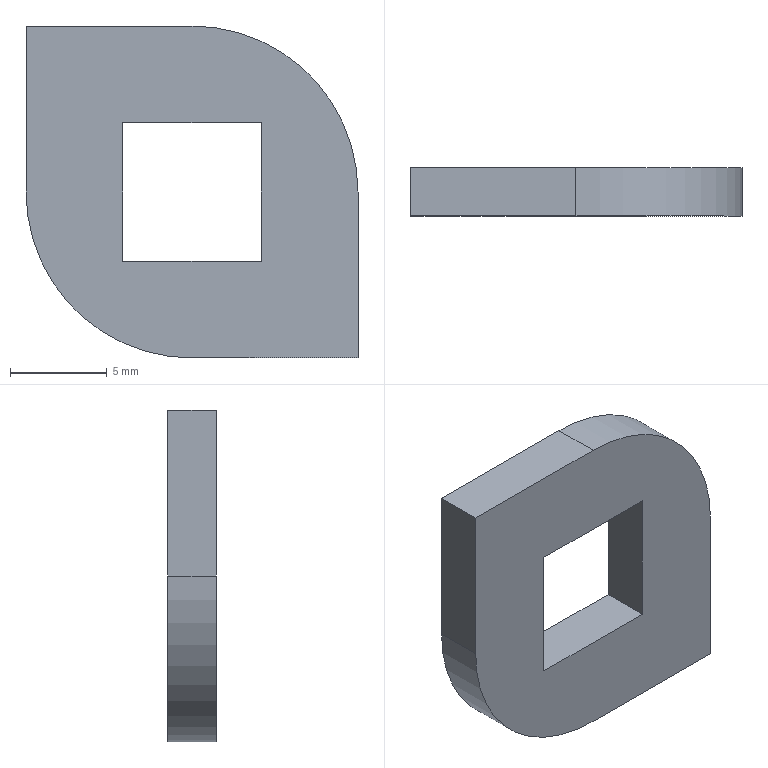Part | STEP file | _X2_751F4E45_X0_MS731-1_X2_8F_4 | 1 solid | 12 faces | box 17.2 x 2.5 x 17.2 mm | volume 530.64 mm3 | plane 10 | cylinder 2 | commonest cylinder face diameters 17.2 x2
STEP:
#1=CARTESIAN_POINT('',(0.,0.,0.));
#2=DIRECTION('',(0.,0.,1.));
#3=DIRECTION('',(1.,0.,0.));
#4=AXIS2_PLACEMENT_3D('',#1,#2,#3);
#5=CARTESIAN_POINT('',(15.5,-5.619,-117.1));
#6=VERTEX_POINT('',#5);
#7=CARTESIAN_POINT('',(24.1,-5.619,-117.1));
#8=VERTEX_POINT('',#7);
#9=CARTESIAN_POINT('',(15.5,-5.619,-117.1));
#10=DIRECTION('',(1.,0.,0.));
#11=VECTOR('',#10,1.);
#12=LINE('',#9,#11);
#13=CARTESIAN_POINT('',(15.5,-5.619,-108.5));
#14=DIRECTION('',(0.,1.,0.));
#15=DIRECTION('',(-1.,0.,0.));
#16=AXIS2_PLACEMENT_3D('',#13,#14,#15);
#17=PLANE('',#16);
#18=CARTESIAN_POINT('',(0.,-8.6));
#19=DIRECTION('',(-1.,0.));
#20=VECTOR('',#19,1.);
#21=LINE('',#18,#20);
#22=(GEOMETRIC_REPRESENTATION_CONTEXT(2)PARAMETRIC_REPRESENTATION_CONTEXT()REPRESENTATION_CONTEXT('',''));
#23=DEFINITIONAL_REPRESENTATION('',(#21),#22);
#24=PCURVE('',#17,#23);
#25=CARTESIAN_POINT('',(24.1,-5.619,-117.1));
#26=DIRECTION('',(0.,0.,-1.));
#27=DIRECTION('',(1.,0.,0.));
#28=AXIS2_PLACEMENT_3D('',#25,#26,#27);
#29=PLANE('',#28);
#30=CARTESIAN_POINT('',(-8.6,0.));
#31=DIRECTION('',(1.,0.));
#32=VECTOR('',#31,1.);
#33=LINE('',#30,#32);
#34=(GEOMETRIC_REPRESENTATION_CONTEXT(2)PARAMETRIC_REPRESENTATION_CONTEXT()REPRESENTATION_CONTEXT('',''));
#35=DEFINITIONAL_REPRESENTATION('',(#33),#34);
#36=PCURVE('',#29,#35);
#37=SURFACE_CURVE('',#12,(#24,#36),.PCURVE_S1.);
#38=EDGE_CURVE('',#6,#8,#37,.T.);
#39=ORIENTED_EDGE('',*,*,#38,.F.);
#40=CARTESIAN_POINT('',(6.9,-5.619,-108.5));
#41=VERTEX_POINT('',#40);
#42=CARTESIAN_POINT('',(15.5,-5.619,-108.5));
#43=DIRECTION('',(0.,-1.,0.));
#44=DIRECTION('',(-1.,0.,0.));
#45=AXIS2_PLACEMENT_3D('',#42,#43,#44);
#46=CIRCLE('',#45,8.6);
#47=CARTESIAN_POINT('',(8.6,0.));
#48=CARTESIAN_POINT('',(8.6,-14.896));
#49=CARTESIAN_POINT('',(-4.3,-7.448));
#50=CARTESIAN_POINT('',(-17.2,0.));
#51=CARTESIAN_POINT('',(-4.3,7.448));
#52=CARTESIAN_POINT('',(8.6,14.896));
#53=CARTESIAN_POINT('',(8.6,0.));
#54=(BOUNDED_CURVE()B_SPLINE_CURVE(2,(#47,#48,#49,#50,#51,#52,#53),.UNSPECIFIED.,.T.,.F.)B_SPLINE_CURVE_WITH_KNOTS((1,2,2,2,2,1),(-2.094,0.,2.094,4.189,6.283,8.378),.UNSPECIFIED.)CURVE()GEOMETRIC_REPRESENTATION_ITEM()RATIONAL_B_SPLINE_CURVE((1.,0.5,1.,0.5,1.,0.5,1.))REPRESENTATION_ITEM(''));
#55=(GEOMETRIC_REPRESENTATION_CONTEXT(2)PARAMETRIC_REPRESENTATION_CONTEXT()REPRESENTATION_CONTEXT('',''));
#56=DEFINITIONAL_REPRESENTATION('',(#54),#55);
#57=PCURVE('',#17,#56);
#58=CARTESIAN_POINT('',(15.5,-5.619,-108.5));
#59=DIRECTION('',(0.,1.,0.));
#60=DIRECTION('',(-1.,0.,0.));
#61=AXIS2_PLACEMENT_3D('',#58,#59,#60);
#62=CYLINDRICAL_SURFACE('',#61,8.6);
#63=CARTESIAN_POINT('',(6.283,0.));
#64=DIRECTION('',(-1.,0.));
#65=VECTOR('',#64,1.);
#66=LINE('',#63,#65);
#67=(GEOMETRIC_REPRESENTATION_CONTEXT(2)PARAMETRIC_REPRESENTATION_CONTEXT()REPRESENTATION_CONTEXT('',''));
#68=DEFINITIONAL_REPRESENTATION('',(#66),#67);
#69=PCURVE('',#62,#68);
#70=SURFACE_CURVE('',#46,(#57,#69),.PCURVE_S1.);
#71=EDGE_CURVE('',#41,#6,#70,.T.);
#72=ORIENTED_EDGE('',*,*,#71,.F.);
#73=CARTESIAN_POINT('',(6.9,-5.619,-99.9));
#74=VERTEX_POINT('',#73);
#75=CARTESIAN_POINT('',(6.9,-5.619,-99.9));
#76=DIRECTION('',(0.,0.,-1.));
#77=VECTOR('',#76,1.);
#78=LINE('',#75,#77);
#79=CARTESIAN_POINT('',(8.6,8.6));
#80=DIRECTION('',(0.,-1.));
#81=VECTOR('',#80,1.);
#82=LINE('',#79,#81);
#83=(GEOMETRIC_REPRESENTATION_CONTEXT(2)PARAMETRIC_REPRESENTATION_CONTEXT()REPRESENTATION_CONTEXT('',''));
#84=DEFINITIONAL_REPRESENTATION('',(#82),#83);
#85=PCURVE('',#17,#84);
#86=CARTESIAN_POINT('',(6.9,-5.619,-108.5));
#87=DIRECTION('',(-1.,0.,0.));
#88=DIRECTION('',(0.,0.,-1.));
#89=AXIS2_PLACEMENT_3D('',#86,#87,#88);
#90=PLANE('',#89);
#91=CARTESIAN_POINT('',(-8.6,0.));
#92=DIRECTION('',(1.,0.));
#93=VECTOR('',#92,1.);
#94=LINE('',#91,#93);
#95=(GEOMETRIC_REPRESENTATION_CONTEXT(2)PARAMETRIC_REPRESENTATION_CONTEXT()REPRESENTATION_CONTEXT('',''));
#96=DEFINITIONAL_REPRESENTATION('',(#94),#95);
#97=PCURVE('',#90,#96);
#98=SURFACE_CURVE('',#78,(#85,#97),.PCURVE_S1.);
#99=EDGE_CURVE('',#74,#41,#98,.T.);
#100=ORIENTED_EDGE('',*,*,#99,.F.);
#101=CARTESIAN_POINT('',(15.5,-5.619,-99.9));
#102=VERTEX_POINT('',#101);
#103=CARTESIAN_POINT('',(15.5,-5.619,-99.9));
#104=DIRECTION('',(-1.,0.,0.));
#105=VECTOR('',#104,1.);
#106=LINE('',#103,#105);
#107=CARTESIAN_POINT('',(0.,8.6));
#108=DIRECTION('',(1.,0.));
#109=VECTOR('',#108,1.);
#110=LINE('',#107,#109);
#111=(GEOMETRIC_REPRESENTATION_CONTEXT(2)PARAMETRIC_REPRESENTATION_CONTEXT()REPRESENTATION_CONTEXT('',''));
#112=DEFINITIONAL_REPRESENTATION('',(#110),#111);
#113=PCURVE('',#17,#112);
#114=CARTESIAN_POINT('',(6.9,-5.619,-99.9));
#115=DIRECTION('',(0.,0.,1.));
#116=DIRECTION('',(-1.,0.,0.));
#117=AXIS2_PLACEMENT_3D('',#114,#115,#116);
#118=PLANE('',#117);
#119=CARTESIAN_POINT('',(-8.6,0.));
#120=DIRECTION('',(1.,0.));
#121=VECTOR('',#120,1.);
#122=LINE('',#119,#121);
#123=(GEOMETRIC_REPRESENTATION_CONTEXT(2)PARAMETRIC_REPRESENTATION_CONTEXT()REPRESENTATION_CONTEXT('',''));
#124=DEFINITIONAL_REPRESENTATION('',(#122),#123);
#125=PCURVE('',#118,#124);
#126=SURFACE_CURVE('',#106,(#113,#125),.PCURVE_S1.);
#127=EDGE_CURVE('',#102,#74,#126,.T.);
#128=ORIENTED_EDGE('',*,*,#127,.F.);
#129=CARTESIAN_POINT('',(24.1,-5.619,-108.5));
#130=VERTEX_POINT('',#129);
#131=CARTESIAN_POINT('',(15.5,-5.619,-108.5));
#132=DIRECTION('',(0.,-1.,0.));
#133=DIRECTION('',(1.,0.,0.));
#134=AXIS2_PLACEMENT_3D('',#131,#132,#133);
#135=CIRCLE('',#134,8.6);
#136=CARTESIAN_POINT('',(-8.6,0.));
#137=CARTESIAN_POINT('',(-8.6,14.896));
#138=CARTESIAN_POINT('',(4.3,7.448));
#139=CARTESIAN_POINT('',(17.2,0.));
#140=CARTESIAN_POINT('',(4.3,-7.448));
#141=CARTESIAN_POINT('',(-8.6,-14.896));
#142=CARTESIAN_POINT('',(-8.6,0.));
#143=(BOUNDED_CURVE()B_SPLINE_CURVE(2,(#136,#137,#138,#139,#140,#141,#142),.UNSPECIFIED.,.T.,.F.)B_SPLINE_CURVE_WITH_KNOTS((1,2,2,2,2,1),(-2.094,0.,2.094,4.189,6.283,8.378),.UNSPECIFIED.)CURVE()GEOMETRIC_REPRESENTATION_ITEM()RATIONAL_B_SPLINE_CURVE((1.,0.5,1.,0.5,1.,0.5,1.))REPRESENTATION_ITEM(''));
#144=(GEOMETRIC_REPRESENTATION_CONTEXT(2)PARAMETRIC_REPRESENTATION_CONTEXT()REPRESENTATION_CONTEXT('',''));
#145=DEFINITIONAL_REPRESENTATION('',(#143),#144);
#146=PCURVE('',#17,#145);
#147=CARTESIAN_POINT('',(15.5,-5.619,-108.5));
#148=DIRECTION('',(0.,1.,0.));
#149=DIRECTION('',(-1.,0.,0.));
#150=AXIS2_PLACEMENT_3D('',#147,#148,#149);
#151=CYLINDRICAL_SURFACE('',#150,8.6);
#152=CARTESIAN_POINT('',(3.142,0.));
#153=DIRECTION('',(-1.,0.));
#154=VECTOR('',#153,1.);
#155=LINE('',#152,#154);
#156=(GEOMETRIC_REPRESENTATION_CONTEXT(2)PARAMETRIC_REPRESENTATION_CONTEXT()REPRESENTATION_CONTEXT('',''));
#157=DEFINITIONAL_REPRESENTATION('',(#155),#156);
#158=PCURVE('',#151,#157);
#159=SURFACE_CURVE('',#135,(#146,#158),.PCURVE_S1.);
#160=EDGE_CURVE('',#130,#102,#159,.T.);
#161=ORIENTED_EDGE('',*,*,#160,.F.);
#162=CARTESIAN_POINT('',(24.1,-5.619,-117.1));
#163=DIRECTION('',(0.,0.,1.));
#164=VECTOR('',#163,1.);
#165=LINE('',#162,#164);
#166=CARTESIAN_POINT('',(-8.6,-8.6));
#167=DIRECTION('',(0.,1.));
#168=VECTOR('',#167,1.);
#169=LINE('',#166,#168);
#170=(GEOMETRIC_REPRESENTATION_CONTEXT(2)PARAMETRIC_REPRESENTATION_CONTEXT()REPRESENTATION_CONTEXT('',''));
#171=DEFINITIONAL_REPRESENTATION('',(#169),#170);
#172=PCURVE('',#17,#171);
#173=CARTESIAN_POINT('',(24.1,-5.619,-108.5));
#174=DIRECTION('',(1.,0.,0.));
#175=DIRECTION('',(0.,0.,1.));
#176=AXIS2_PLACEMENT_3D('',#173,#174,#175);
#177=PLANE('',#176);
#178=CARTESIAN_POINT('',(-8.6,0.));
#179=DIRECTION('',(1.,0.));
#180=VECTOR('',#179,1.);
#181=LINE('',#178,#180);
#182=(GEOMETRIC_REPRESENTATION_CONTEXT(2)PARAMETRIC_REPRESENTATION_CONTEXT()REPRESENTATION_CONTEXT('',''));
#183=DEFINITIONAL_REPRESENTATION('',(#181),#182);
#184=PCURVE('',#177,#183);
#185=SURFACE_CURVE('',#165,(#172,#184),.PCURVE_S1.);
#186=EDGE_CURVE('',#8,#130,#185,.T.);
#187=ORIENTED_EDGE('',*,*,#186,.F.);
#188=EDGE_LOOP('',(#39,#72,#100,#128,#161,#187));
#189=FACE_BOUND('',#188,.F.);
#190=CARTESIAN_POINT('',(11.9,-5.619,-104.9));
#191=VERTEX_POINT('',#190);
#192=CARTESIAN_POINT('',(19.1,-5.619,-104.9));
#193=VERTEX_POINT('',#192);
#194=CARTESIAN_POINT('',(11.9,-5.619,-104.9));
#195=DIRECTION('',(1.,0.,0.));
#196=VECTOR('',#195,1.);
#197=LINE('',#194,#196);
#198=CARTESIAN_POINT('',(3.6,3.6));
#199=DIRECTION('',(-1.,0.));
#200=VECTOR('',#199,1.);
#201=LINE('',#198,#200);
#202=(GEOMETRIC_REPRESENTATION_CONTEXT(2)PARAMETRIC_REPRESENTATION_CONTEXT()REPRESENTATION_CONTEXT('',''));
#203=DEFINITIONAL_REPRESENTATION('',(#201),#202);
#204=PCURVE('',#17,#203);
#205=CARTESIAN_POINT('',(19.1,-5.619,-104.9));
#206=DIRECTION('',(0.,0.,-1.));
#207=DIRECTION('',(1.,0.,0.));
#208=AXIS2_PLACEMENT_3D('',#205,#206,#207);
#209=PLANE('',#208);
#210=CARTESIAN_POINT('',(-7.2,0.));
#211=DIRECTION('',(1.,0.));
#212=VECTOR('',#211,1.);
#213=LINE('',#210,#212);
#214=(GEOMETRIC_REPRESENTATION_CONTEXT(2)PARAMETRIC_REPRESENTATION_CONTEXT()REPRESENTATION_CONTEXT('',''));
#215=DEFINITIONAL_REPRESENTATION('',(#213),#214);
#216=PCURVE('',#209,#215);
#217=SURFACE_CURVE('',#197,(#204,#216),.PCURVE_S1.);
#218=EDGE_CURVE('',#191,#193,#217,.T.);
#219=ORIENTED_EDGE('',*,*,#218,.F.);
#220=CARTESIAN_POINT('',(11.9,-5.619,-112.1));
#221=VERTEX_POINT('',#220);
#222=CARTESIAN_POINT('',(11.9,-5.619,-112.1));
#223=DIRECTION('',(0.,0.,1.));
#224=VECTOR('',#223,1.);
#225=LINE('',#222,#224);
#226=CARTESIAN_POINT('',(3.6,-3.6));
#227=DIRECTION('',(0.,1.));
#228=VECTOR('',#227,1.);
#229=LINE('',#226,#228);
#230=(GEOMETRIC_REPRESENTATION_CONTEXT(2)PARAMETRIC_REPRESENTATION_CONTEXT()REPRESENTATION_CONTEXT('',''));
#231=DEFINITIONAL_REPRESENTATION('',(#229),#230);
#232=PCURVE('',#17,#231);
#233=CARTESIAN_POINT('',(11.9,-5.619,-104.9));
#234=DIRECTION('',(1.,0.,0.));
#235=DIRECTION('',(0.,0.,1.));
#236=AXIS2_PLACEMENT_3D('',#233,#234,#235);
#237=PLANE('',#236);
#238=CARTESIAN_POINT('',(-7.2,0.));
#239=DIRECTION('',(1.,0.));
#240=VECTOR('',#239,1.);
#241=LINE('',#238,#240);
#242=(GEOMETRIC_REPRESENTATION_CONTEXT(2)PARAMETRIC_REPRESENTATION_CONTEXT()REPRESENTATION_CONTEXT('',''));
#243=DEFINITIONAL_REPRESENTATION('',(#241),#242);
#244=PCURVE('',#237,#243);
#245=SURFACE_CURVE('',#225,(#232,#244),.PCURVE_S1.);
#246=EDGE_CURVE('',#221,#191,#245,.T.);
#247=ORIENTED_EDGE('',*,*,#246,.F.);
#248=CARTESIAN_POINT('',(19.1,-5.619,-112.1));
#249=VERTEX_POINT('',#248);
#250=CARTESIAN_POINT('',(19.1,-5.619,-112.1));
#251=DIRECTION('',(-1.,0.,0.));
#252=VECTOR('',#251,1.);
#253=LINE('',#250,#252);
#254=CARTESIAN_POINT('',(-3.6,-3.6));
#255=DIRECTION('',(1.,0.));
#256=VECTOR('',#255,1.);
#257=LINE('',#254,#256);
#258=(GEOMETRIC_REPRESENTATION_CONTEXT(2)PARAMETRIC_REPRESENTATION_CONTEXT()REPRESENTATION_CONTEXT('',''));
#259=DEFINITIONAL_REPRESENTATION('',(#257),#258);
#260=PCURVE('',#17,#259);
#261=CARTESIAN_POINT('',(11.9,-5.619,-112.1));
#262=DIRECTION('',(0.,0.,1.));
#263=DIRECTION('',(-1.,0.,0.));
#264=AXIS2_PLACEMENT_3D('',#261,#262,#263);
#265=PLANE('',#264);
#266=CARTESIAN_POINT('',(-7.2,0.));
#267=DIRECTION('',(1.,0.));
#268=VECTOR('',#267,1.);
#269=LINE('',#266,#268);
#270=(GEOMETRIC_REPRESENTATION_CONTEXT(2)PARAMETRIC_REPRESENTATION_CONTEXT()REPRESENTATION_CONTEXT('',''));
#271=DEFINITIONAL_REPRESENTATION('',(#269),#270);
#272=PCURVE('',#265,#271);
#273=SURFACE_CURVE('',#253,(#260,#272),.PCURVE_S1.);
#274=EDGE_CURVE('',#249,#221,#273,.T.);
#275=ORIENTED_EDGE('',*,*,#274,.F.);
#276=CARTESIAN_POINT('',(19.1,-5.619,-104.9));
#277=DIRECTION('',(0.,0.,-1.));
#278=VECTOR('',#277,1.);
#279=LINE('',#276,#278);
#280=CARTESIAN_POINT('',(-3.6,3.6));
#281=DIRECTION('',(0.,-1.));
#282=VECTOR('',#281,1.);
#283=LINE('',#280,#282);
#284=(GEOMETRIC_REPRESENTATION_CONTEXT(2)PARAMETRIC_REPRESENTATION_CONTEXT()REPRESENTATION_CONTEXT('',''));
#285=DEFINITIONAL_REPRESENTATION('',(#283),#284);
#286=PCURVE('',#17,#285);
#287=CARTESIAN_POINT('',(19.1,-5.619,-112.1));
#288=DIRECTION('',(-1.,0.,0.));
#289=DIRECTION('',(0.,0.,-1.));
#290=AXIS2_PLACEMENT_3D('',#287,#288,#289);
#291=PLANE('',#290);
#292=CARTESIAN_POINT('',(-7.2,0.));
#293=DIRECTION('',(1.,0.));
#294=VECTOR('',#293,1.);
#295=LINE('',#292,#294);
#296=(GEOMETRIC_REPRESENTATION_CONTEXT(2)PARAMETRIC_REPRESENTATION_CONTEXT()REPRESENTATION_CONTEXT('',''));
#297=DEFINITIONAL_REPRESENTATION('',(#295),#296);
#298=PCURVE('',#291,#297);
#299=SURFACE_CURVE('',#279,(#286,#298),.PCURVE_S1.);
#300=EDGE_CURVE('',#193,#249,#299,.T.);
#301=ORIENTED_EDGE('',*,*,#300,.F.);
#302=EDGE_LOOP('',(#219,#247,#275,#301));
#303=FACE_BOUND('',#302,.F.);
#304=ADVANCED_FACE('',(#189,#303),#17,.F.);
#305=CARTESIAN_POINT('',(15.5,-3.119,-117.1));
#306=VERTEX_POINT('',#305);
#307=CARTESIAN_POINT('',(15.5,-3.119,-117.1));
#308=DIRECTION('',(0.,-1.,0.));
#309=VECTOR('',#308,1.);
#310=LINE('',#307,#309);
#311=CARTESIAN_POINT('',(-8.6,-2.5));
#312=DIRECTION('',(0.,1.));
#313=VECTOR('',#312,1.);
#314=LINE('',#311,#313);
#315=(GEOMETRIC_REPRESENTATION_CONTEXT(2)PARAMETRIC_REPRESENTATION_CONTEXT()REPRESENTATION_CONTEXT('',''));
#316=DEFINITIONAL_REPRESENTATION('',(#314),#315);
#317=PCURVE('',#29,#316);
#318=CARTESIAN_POINT('',(4.712,2.5));
#319=DIRECTION('',(0.,-1.));
#320=VECTOR('',#319,1.);
#321=LINE('',#318,#320);
#322=(GEOMETRIC_REPRESENTATION_CONTEXT(2)PARAMETRIC_REPRESENTATION_CONTEXT()REPRESENTATION_CONTEXT('',''));
#323=DEFINITIONAL_REPRESENTATION('',(#321),#322);
#324=PCURVE('',#62,#323);
#325=SURFACE_CURVE('',#310,(#317,#324),.PCURVE_S1.);
#326=EDGE_CURVE('',#306,#6,#325,.T.);
#327=ORIENTED_EDGE('',*,*,#326,.T.);
#328=ORIENTED_EDGE('',*,*,#38,.T.);
#329=CARTESIAN_POINT('',(24.1,-3.119,-117.1));
#330=VERTEX_POINT('',#329);
#331=CARTESIAN_POINT('',(24.1,-3.119,-117.1));
#332=DIRECTION('',(0.,-1.,0.));
#333=VECTOR('',#332,1.);
#334=LINE('',#331,#333);
#335=CARTESIAN_POINT('',(0.,-2.5));
#336=DIRECTION('',(0.,1.));
#337=VECTOR('',#336,1.);
#338=LINE('',#335,#337);
#339=(GEOMETRIC_REPRESENTATION_CONTEXT(2)PARAMETRIC_REPRESENTATION_CONTEXT()REPRESENTATION_CONTEXT('',''));
#340=DEFINITIONAL_REPRESENTATION('',(#338),#339);
#341=PCURVE('',#29,#340);
#342=CARTESIAN_POINT('',(-8.6,-2.5));
#343=DIRECTION('',(0.,1.));
#344=VECTOR('',#343,1.);
#345=LINE('',#342,#344);
#346=(GEOMETRIC_REPRESENTATION_CONTEXT(2)PARAMETRIC_REPRESENTATION_CONTEXT()REPRESENTATION_CONTEXT('',''));
#347=DEFINITIONAL_REPRESENTATION('',(#345),#346);
#348=PCURVE('',#177,#347);
#349=SURFACE_CURVE('',#334,(#341,#348),.PCURVE_S1.);
#350=EDGE_CURVE('',#330,#8,#349,.T.);
#351=ORIENTED_EDGE('',*,*,#350,.F.);
#352=CARTESIAN_POINT('',(15.5,-3.119,-117.1));
#353=DIRECTION('',(1.,0.,0.));
#354=VECTOR('',#353,1.);
#355=LINE('',#352,#354);
#356=CARTESIAN_POINT('',(-8.6,-2.5));
#357=DIRECTION('',(1.,0.));
#358=VECTOR('',#357,1.);
#359=LINE('',#356,#358);
#360=(GEOMETRIC_REPRESENTATION_CONTEXT(2)PARAMETRIC_REPRESENTATION_CONTEXT()REPRESENTATION_CONTEXT('',''));
#361=DEFINITIONAL_REPRESENTATION('',(#359),#360);
#362=PCURVE('',#29,#361);
#363=CARTESIAN_POINT('',(15.5,-3.119,-108.5));
#364=DIRECTION('',(0.,1.,0.));
#365=DIRECTION('',(-1.,0.,0.));
#366=AXIS2_PLACEMENT_3D('',#363,#364,#365);
#367=PLANE('',#366);
#368=CARTESIAN_POINT('',(0.,-8.6));
#369=DIRECTION('',(-1.,0.));
#370=VECTOR('',#369,1.);
#371=LINE('',#368,#370);
#372=(GEOMETRIC_REPRESENTATION_CONTEXT(2)PARAMETRIC_REPRESENTATION_CONTEXT()REPRESENTATION_CONTEXT('',''));
#373=DEFINITIONAL_REPRESENTATION('',(#371),#372);
#374=PCURVE('',#367,#373);
#375=SURFACE_CURVE('',#355,(#362,#374),.PCURVE_S1.);
#376=EDGE_CURVE('',#306,#330,#375,.T.);
#377=ORIENTED_EDGE('',*,*,#376,.F.);
#378=EDGE_LOOP('',(#327,#328,#351,#377));
#379=FACE_BOUND('',#378,.F.);
#380=ADVANCED_FACE('',(#379),#29,.T.);
#381=CARTESIAN_POINT('',(6.9,-3.119,-108.5));
#382=VERTEX_POINT('',#381);
#383=CARTESIAN_POINT('',(15.5,-3.119,-108.5));
#384=DIRECTION('',(0.,1.,0.));
#385=DIRECTION('',(0.,0.,-1.));
#386=AXIS2_PLACEMENT_3D('',#383,#384,#385);
#387=CIRCLE('',#386,8.6);
#388=CARTESIAN_POINT('',(4.712,2.5));
#389=DIRECTION('',(1.,0.));
#390=VECTOR('',#389,1.);
#391=LINE('',#388,#390);
#392=(GEOMETRIC_REPRESENTATION_CONTEXT(2)PARAMETRIC_REPRESENTATION_CONTEXT()REPRESENTATION_CONTEXT('',''));
#393=DEFINITIONAL_REPRESENTATION('',(#391),#392);
#394=PCURVE('',#62,#393);
#395=CARTESIAN_POINT('',(0.,0.));
#396=DIRECTION('',(0.,-1.));
#397=AXIS2_PLACEMENT_2D('',#395,#396);
#398=CIRCLE('',#397,8.6);
#399=(GEOMETRIC_REPRESENTATION_CONTEXT(2)PARAMETRIC_REPRESENTATION_CONTEXT()REPRESENTATION_CONTEXT('',''));
#400=DEFINITIONAL_REPRESENTATION('',(#398),#399);
#401=PCURVE('',#367,#400);
#402=SURFACE_CURVE('',#387,(#394,#401),.PCURVE_S1.);
#403=EDGE_CURVE('',#306,#382,#402,.T.);
#404=ORIENTED_EDGE('',*,*,#403,.F.);
#405=ORIENTED_EDGE('',*,*,#326,.T.);
#406=ORIENTED_EDGE('',*,*,#71,.F.);
#407=CARTESIAN_POINT('',(6.9,-5.619,-108.5));
#408=DIRECTION('',(0.,1.,0.));
#409=VECTOR('',#408,1.);
#410=LINE('',#407,#409);
#411=CARTESIAN_POINT('',(6.283,0.));
#412=DIRECTION('',(0.,1.));
#413=VECTOR('',#412,1.);
#414=LINE('',#411,#413);
#415=(GEOMETRIC_REPRESENTATION_CONTEXT(2)PARAMETRIC_REPRESENTATION_CONTEXT()REPRESENTATION_CONTEXT('',''));
#416=DEFINITIONAL_REPRESENTATION('',(#414),#415);
#417=PCURVE('',#62,#416);
#418=CARTESIAN_POINT('',(0.,0.));
#419=DIRECTION('',(0.,-1.));
#420=VECTOR('',#419,1.);
#421=LINE('',#418,#420);
#422=(GEOMETRIC_REPRESENTATION_CONTEXT(2)PARAMETRIC_REPRESENTATION_CONTEXT()REPRESENTATION_CONTEXT('',''));
#423=DEFINITIONAL_REPRESENTATION('',(#421),#422);
#424=PCURVE('',#90,#423);
#425=SURFACE_CURVE('',#410,(#417,#424),.PCURVE_S1.);
#426=EDGE_CURVE('',#41,#382,#425,.T.);
#427=ORIENTED_EDGE('',*,*,#426,.T.);
#428=EDGE_LOOP('',(#404,#405,#406,#427));
#429=FACE_BOUND('',#428,.T.);
#430=ADVANCED_FACE('',(#429),#62,.T.);
#431=CARTESIAN_POINT('',(6.9,-3.119,-99.9));
#432=VERTEX_POINT('',#431);
#433=CARTESIAN_POINT('',(6.9,-3.119,-99.9));
#434=DIRECTION('',(0.,-1.,0.));
#435=VECTOR('',#434,1.);
#436=LINE('',#433,#435);
#437=CARTESIAN_POINT('',(-8.6,-2.5));
#438=DIRECTION('',(0.,1.));
#439=VECTOR('',#438,1.);
#440=LINE('',#437,#439);
#441=(GEOMETRIC_REPRESENTATION_CONTEXT(2)PARAMETRIC_REPRESENTATION_CONTEXT()REPRESENTATION_CONTEXT('',''));
#442=DEFINITIONAL_REPRESENTATION('',(#440),#441);
#443=PCURVE('',#90,#442);
#444=CARTESIAN_POINT('',(0.,-2.5));
#445=DIRECTION('',(0.,1.));
#446=VECTOR('',#445,1.);
#447=LINE('',#444,#446);
#448=(GEOMETRIC_REPRESENTATION_CONTEXT(2)PARAMETRIC_REPRESENTATION_CONTEXT()REPRESENTATION_CONTEXT('',''));
#449=DEFINITIONAL_REPRESENTATION('',(#447),#448);
#450=PCURVE('',#118,#449);
#451=SURFACE_CURVE('',#436,(#443,#450),.PCURVE_S1.);
#452=EDGE_CURVE('',#432,#74,#451,.T.);
#453=ORIENTED_EDGE('',*,*,#452,.T.);
#454=ORIENTED_EDGE('',*,*,#99,.T.);
#455=ORIENTED_EDGE('',*,*,#426,.T.);
#456=CARTESIAN_POINT('',(6.9,-3.119,-99.9));
#457=DIRECTION('',(0.,0.,-1.));
#458=VECTOR('',#457,1.);
#459=LINE('',#456,#458);
#460=CARTESIAN_POINT('',(-8.6,-2.5));
#461=DIRECTION('',(1.,0.));
#462=VECTOR('',#461,1.);
#463=LINE('',#460,#462);
#464=(GEOMETRIC_REPRESENTATION_CONTEXT(2)PARAMETRIC_REPRESENTATION_CONTEXT()REPRESENTATION_CONTEXT('',''));
#465=DEFINITIONAL_REPRESENTATION('',(#463),#464);
#466=PCURVE('',#90,#465);
#467=CARTESIAN_POINT('',(8.6,8.6));
#468=DIRECTION('',(0.,-1.));
#469=VECTOR('',#468,1.);
#470=LINE('',#467,#469);
#471=(GEOMETRIC_REPRESENTATION_CONTEXT(2)PARAMETRIC_REPRESENTATION_CONTEXT()REPRESENTATION_CONTEXT('',''));
#472=DEFINITIONAL_REPRESENTATION('',(#470),#471);
#473=PCURVE('',#367,#472);
#474=SURFACE_CURVE('',#459,(#466,#473),.PCURVE_S1.);
#475=EDGE_CURVE('',#432,#382,#474,.T.);
#476=ORIENTED_EDGE('',*,*,#475,.F.);
#477=EDGE_LOOP('',(#453,#454,#455,#476));
#478=FACE_BOUND('',#477,.F.);
#479=ADVANCED_FACE('',(#478),#90,.T.);
#480=CARTESIAN_POINT('',(15.5,-3.119,-99.9));
#481=VERTEX_POINT('',#480);
#482=CARTESIAN_POINT('',(15.5,-3.119,-99.9));
#483=DIRECTION('',(0.,-1.,0.));
#484=VECTOR('',#483,1.);
#485=LINE('',#482,#484);
#486=CARTESIAN_POINT('',(-8.6,-2.5));
#487=DIRECTION('',(0.,1.));
#488=VECTOR('',#487,1.);
#489=LINE('',#486,#488);
#490=(GEOMETRIC_REPRESENTATION_CONTEXT(2)PARAMETRIC_REPRESENTATION_CONTEXT()REPRESENTATION_CONTEXT('',''));
#491=DEFINITIONAL_REPRESENTATION('',(#489),#490);
#492=PCURVE('',#118,#491);
#493=CARTESIAN_POINT('',(1.571,2.5));
#494=DIRECTION('',(0.,-1.));
#495=VECTOR('',#494,1.);
#496=LINE('',#493,#495);
#497=(GEOMETRIC_REPRESENTATION_CONTEXT(2)PARAMETRIC_REPRESENTATION_CONTEXT()REPRESENTATION_CONTEXT('',''));
#498=DEFINITIONAL_REPRESENTATION('',(#496),#497);
#499=PCURVE('',#151,#498);
#500=SURFACE_CURVE('',#485,(#492,#499),.PCURVE_S1.);
#501=EDGE_CURVE('',#481,#102,#500,.T.);
#502=ORIENTED_EDGE('',*,*,#501,.T.);
#503=ORIENTED_EDGE('',*,*,#127,.T.);
#504=ORIENTED_EDGE('',*,*,#452,.F.);
#505=CARTESIAN_POINT('',(15.5,-3.119,-99.9));
#506=DIRECTION('',(-1.,0.,0.));
#507=VECTOR('',#506,1.);
#508=LINE('',#505,#507);
#509=CARTESIAN_POINT('',(-8.6,-2.5));
#510=DIRECTION('',(1.,0.));
#511=VECTOR('',#510,1.);
#512=LINE('',#509,#511);
#513=(GEOMETRIC_REPRESENTATION_CONTEXT(2)PARAMETRIC_REPRESENTATION_CONTEXT()REPRESENTATION_CONTEXT('',''));
#514=DEFINITIONAL_REPRESENTATION('',(#512),#513);
#515=PCURVE('',#118,#514);
#516=CARTESIAN_POINT('',(0.,8.6));
#517=DIRECTION('',(1.,0.));
#518=VECTOR('',#517,1.);
#519=LINE('',#516,#518);
#520=(GEOMETRIC_REPRESENTATION_CONTEXT(2)PARAMETRIC_REPRESENTATION_CONTEXT()REPRESENTATION_CONTEXT('',''));
#521=DEFINITIONAL_REPRESENTATION('',(#519),#520);
#522=PCURVE('',#367,#521);
#523=SURFACE_CURVE('',#508,(#515,#522),.PCURVE_S1.);
#524=EDGE_CURVE('',#481,#432,#523,.T.);
#525=ORIENTED_EDGE('',*,*,#524,.F.);
#526=EDGE_LOOP('',(#502,#503,#504,#525));
#527=FACE_BOUND('',#526,.F.);
#528=ADVANCED_FACE('',(#527),#118,.T.);
#529=CARTESIAN_POINT('',(24.1,-3.119,-108.5));
#530=VERTEX_POINT('',#529);
#531=CARTESIAN_POINT('',(15.5,-3.119,-108.5));
#532=DIRECTION('',(0.,1.,0.));
#533=DIRECTION('',(0.,0.,1.));
#534=AXIS2_PLACEMENT_3D('',#531,#532,#533);
#535=CIRCLE('',#534,8.6);
#536=CARTESIAN_POINT('',(1.571,2.5));
#537=DIRECTION('',(1.,0.));
#538=VECTOR('',#537,1.);
#539=LINE('',#536,#538);
#540=(GEOMETRIC_REPRESENTATION_CONTEXT(2)PARAMETRIC_REPRESENTATION_CONTEXT()REPRESENTATION_CONTEXT('',''));
#541=DEFINITIONAL_REPRESENTATION('',(#539),#540);
#542=PCURVE('',#151,#541);
#543=CARTESIAN_POINT('',(0.,0.));
#544=DIRECTION('',(0.,1.));
#545=AXIS2_PLACEMENT_2D('',#543,#544);
#546=CIRCLE('',#545,8.6);
#547=(GEOMETRIC_REPRESENTATION_CONTEXT(2)PARAMETRIC_REPRESENTATION_CONTEXT()REPRESENTATION_CONTEXT('',''));
#548=DEFINITIONAL_REPRESENTATION('',(#546),#547);
#549=PCURVE('',#367,#548);
#550=SURFACE_CURVE('',#535,(#542,#549),.PCURVE_S1.);
#551=EDGE_CURVE('',#481,#530,#550,.T.);
#552=ORIENTED_EDGE('',*,*,#551,.F.);
#553=ORIENTED_EDGE('',*,*,#501,.T.);
#554=ORIENTED_EDGE('',*,*,#160,.F.);
#555=CARTESIAN_POINT('',(24.1,-5.619,-108.5));
#556=DIRECTION('',(0.,1.,0.));
#557=VECTOR('',#556,1.);
#558=LINE('',#555,#557);
#559=CARTESIAN_POINT('',(3.142,0.));
#560=DIRECTION('',(0.,1.));
#561=VECTOR('',#560,1.);
#562=LINE('',#559,#561);
#563=(GEOMETRIC_REPRESENTATION_CONTEXT(2)PARAMETRIC_REPRESENTATION_CONTEXT()REPRESENTATION_CONTEXT('',''));
#564=DEFINITIONAL_REPRESENTATION('',(#562),#563);
#565=PCURVE('',#151,#564);
#566=CARTESIAN_POINT('',(0.,0.));
#567=DIRECTION('',(0.,-1.));
#568=VECTOR('',#567,1.);
#569=LINE('',#566,#568);
#570=(GEOMETRIC_REPRESENTATION_CONTEXT(2)PARAMETRIC_REPRESENTATION_CONTEXT()REPRESENTATION_CONTEXT('',''));
#571=DEFINITIONAL_REPRESENTATION('',(#569),#570);
#572=PCURVE('',#177,#571);
#573=SURFACE_CURVE('',#558,(#565,#572),.PCURVE_S1.);
#574=EDGE_CURVE('',#130,#530,#573,.T.);
#575=ORIENTED_EDGE('',*,*,#574,.T.);
#576=EDGE_LOOP('',(#552,#553,#554,#575));
#577=FACE_BOUND('',#576,.T.);
#578=ADVANCED_FACE('',(#577),#151,.T.);
#579=ORIENTED_EDGE('',*,*,#350,.T.);
#580=ORIENTED_EDGE('',*,*,#186,.T.);
#581=ORIENTED_EDGE('',*,*,#574,.T.);
#582=CARTESIAN_POINT('',(24.1,-3.119,-117.1));
#583=DIRECTION('',(0.,0.,1.));
#584=VECTOR('',#583,1.);
#585=LINE('',#582,#584);
#586=CARTESIAN_POINT('',(-8.6,-2.5));
#587=DIRECTION('',(1.,0.));
#588=VECTOR('',#587,1.);
#589=LINE('',#586,#588);
#590=(GEOMETRIC_REPRESENTATION_CONTEXT(2)PARAMETRIC_REPRESENTATION_CONTEXT()REPRESENTATION_CONTEXT('',''));
#591=DEFINITIONAL_REPRESENTATION('',(#589),#590);
#592=PCURVE('',#177,#591);
#593=CARTESIAN_POINT('',(-8.6,-8.6));
#594=DIRECTION('',(0.,1.));
#595=VECTOR('',#594,1.);
#596=LINE('',#593,#595);
#597=(GEOMETRIC_REPRESENTATION_CONTEXT(2)PARAMETRIC_REPRESENTATION_CONTEXT()REPRESENTATION_CONTEXT('',''));
#598=DEFINITIONAL_REPRESENTATION('',(#596),#597);
#599=PCURVE('',#367,#598);
#600=SURFACE_CURVE('',#585,(#592,#599),.PCURVE_S1.);
#601=EDGE_CURVE('',#330,#530,#600,.T.);
#602=ORIENTED_EDGE('',*,*,#601,.F.);
#603=EDGE_LOOP('',(#579,#580,#581,#602));
#604=FACE_BOUND('',#603,.F.);
#605=ADVANCED_FACE('',(#604),#177,.T.);
#606=ORIENTED_EDGE('',*,*,#475,.T.);
#607=ORIENTED_EDGE('',*,*,#403,.F.);
#608=ORIENTED_EDGE('',*,*,#376,.T.);
#609=ORIENTED_EDGE('',*,*,#601,.T.);
#610=ORIENTED_EDGE('',*,*,#551,.F.);
#611=ORIENTED_EDGE('',*,*,#524,.T.);
#612=EDGE_LOOP('',(#606,#607,#608,#609,#610,#611));
#613=FACE_BOUND('',#612,.F.);
#614=CARTESIAN_POINT('',(19.1,-3.119,-112.1));
#615=VERTEX_POINT('',#614);
#616=CARTESIAN_POINT('',(11.9,-3.119,-112.1));
#617=VERTEX_POINT('',#616);
#618=CARTESIAN_POINT('',(19.1,-3.119,-112.1));
#619=DIRECTION('',(-1.,0.,0.));
#620=VECTOR('',#619,1.);
#621=LINE('',#618,#620);
#622=CARTESIAN_POINT('',(-3.6,-3.6));
#623=DIRECTION('',(1.,0.));
#624=VECTOR('',#623,1.);
#625=LINE('',#622,#624);
#626=(GEOMETRIC_REPRESENTATION_CONTEXT(2)PARAMETRIC_REPRESENTATION_CONTEXT()REPRESENTATION_CONTEXT('',''));
#627=DEFINITIONAL_REPRESENTATION('',(#625),#626);
#628=PCURVE('',#367,#627);
#629=CARTESIAN_POINT('',(-7.2,-2.5));
#630=DIRECTION('',(1.,0.));
#631=VECTOR('',#630,1.);
#632=LINE('',#629,#631);
#633=(GEOMETRIC_REPRESENTATION_CONTEXT(2)PARAMETRIC_REPRESENTATION_CONTEXT()REPRESENTATION_CONTEXT('',''));
#634=DEFINITIONAL_REPRESENTATION('',(#632),#633);
#635=PCURVE('',#265,#634);
#636=SURFACE_CURVE('',#621,(#628,#635),.PCURVE_S1.);
#637=EDGE_CURVE('',#615,#617,#636,.T.);
#638=ORIENTED_EDGE('',*,*,#637,.T.);
#639=CARTESIAN_POINT('',(11.9,-3.119,-104.9));
#640=VERTEX_POINT('',#639);
#641=CARTESIAN_POINT('',(11.9,-3.119,-112.1));
#642=DIRECTION('',(0.,0.,1.));
#643=VECTOR('',#642,1.);
#644=LINE('',#641,#643);
#645=CARTESIAN_POINT('',(3.6,-3.6));
#646=DIRECTION('',(0.,1.));
#647=VECTOR('',#646,1.);
#648=LINE('',#645,#647);
#649=(GEOMETRIC_REPRESENTATION_CONTEXT(2)PARAMETRIC_REPRESENTATION_CONTEXT()REPRESENTATION_CONTEXT('',''));
#650=DEFINITIONAL_REPRESENTATION('',(#648),#649);
#651=PCURVE('',#367,#650);
#652=CARTESIAN_POINT('',(-7.2,-2.5));
#653=DIRECTION('',(1.,0.));
#654=VECTOR('',#653,1.);
#655=LINE('',#652,#654);
#656=(GEOMETRIC_REPRESENTATION_CONTEXT(2)PARAMETRIC_REPRESENTATION_CONTEXT()REPRESENTATION_CONTEXT('',''));
#657=DEFINITIONAL_REPRESENTATION('',(#655),#656);
#658=PCURVE('',#237,#657);
#659=SURFACE_CURVE('',#644,(#651,#658),.PCURVE_S1.);
#660=EDGE_CURVE('',#617,#640,#659,.T.);
#661=ORIENTED_EDGE('',*,*,#660,.T.);
#662=CARTESIAN_POINT('',(19.1,-3.119,-104.9));
#663=VERTEX_POINT('',#662);
#664=CARTESIAN_POINT('',(11.9,-3.119,-104.9));
#665=DIRECTION('',(1.,0.,0.));
#666=VECTOR('',#665,1.);
#667=LINE('',#664,#666);
#668=CARTESIAN_POINT('',(3.6,3.6));
#669=DIRECTION('',(-1.,0.));
#670=VECTOR('',#669,1.);
#671=LINE('',#668,#670);
#672=(GEOMETRIC_REPRESENTATION_CONTEXT(2)PARAMETRIC_REPRESENTATION_CONTEXT()REPRESENTATION_CONTEXT('',''));
#673=DEFINITIONAL_REPRESENTATION('',(#671),#672);
#674=PCURVE('',#367,#673);
#675=CARTESIAN_POINT('',(-7.2,-2.5));
#676=DIRECTION('',(1.,0.));
#677=VECTOR('',#676,1.);
#678=LINE('',#675,#677);
#679=(GEOMETRIC_REPRESENTATION_CONTEXT(2)PARAMETRIC_REPRESENTATION_CONTEXT()REPRESENTATION_CONTEXT('',''));
#680=DEFINITIONAL_REPRESENTATION('',(#678),#679);
#681=PCURVE('',#209,#680);
#682=SURFACE_CURVE('',#667,(#674,#681),.PCURVE_S1.);
#683=EDGE_CURVE('',#640,#663,#682,.T.);
#684=ORIENTED_EDGE('',*,*,#683,.T.);
#685=CARTESIAN_POINT('',(19.1,-3.119,-104.9));
#686=DIRECTION('',(0.,0.,-1.));
#687=VECTOR('',#686,1.);
#688=LINE('',#685,#687);
#689=CARTESIAN_POINT('',(-3.6,3.6));
#690=DIRECTION('',(0.,-1.));
#691=VECTOR('',#690,1.);
#692=LINE('',#689,#691);
#693=(GEOMETRIC_REPRESENTATION_CONTEXT(2)PARAMETRIC_REPRESENTATION_CONTEXT()REPRESENTATION_CONTEXT('',''));
#694=DEFINITIONAL_REPRESENTATION('',(#692),#693);
#695=PCURVE('',#367,#694);
#696=CARTESIAN_POINT('',(-7.2,-2.5));
#697=DIRECTION('',(1.,0.));
#698=VECTOR('',#697,1.);
#699=LINE('',#696,#698);
#700=(GEOMETRIC_REPRESENTATION_CONTEXT(2)PARAMETRIC_REPRESENTATION_CONTEXT()REPRESENTATION_CONTEXT('',''));
#701=DEFINITIONAL_REPRESENTATION('',(#699),#700);
#702=PCURVE('',#291,#701);
#703=SURFACE_CURVE('',#688,(#695,#702),.PCURVE_S1.);
#704=EDGE_CURVE('',#663,#615,#703,.T.);
#705=ORIENTED_EDGE('',*,*,#704,.T.);
#706=EDGE_LOOP('',(#638,#661,#684,#705));
#707=FACE_BOUND('',#706,.F.);
#708=ADVANCED_FACE('',(#613,#707),#367,.T.);
#709=CARTESIAN_POINT('',(19.1,-3.119,-112.1));
#710=DIRECTION('',(0.,-1.,0.));
#711=VECTOR('',#710,1.);
#712=LINE('',#709,#711);
#713=CARTESIAN_POINT('',(-7.2,-2.5));
#714=DIRECTION('',(0.,1.));
#715=VECTOR('',#714,1.);
#716=LINE('',#713,#715);
#717=(GEOMETRIC_REPRESENTATION_CONTEXT(2)PARAMETRIC_REPRESENTATION_CONTEXT()REPRESENTATION_CONTEXT('',''));
#718=DEFINITIONAL_REPRESENTATION('',(#716),#717);
#719=PCURVE('',#265,#718);
#720=CARTESIAN_POINT('',(0.,-2.5));
#721=DIRECTION('',(0.,1.));
#722=VECTOR('',#721,1.);
#723=LINE('',#720,#722);
#724=(GEOMETRIC_REPRESENTATION_CONTEXT(2)PARAMETRIC_REPRESENTATION_CONTEXT()REPRESENTATION_CONTEXT('',''));
#725=DEFINITIONAL_REPRESENTATION('',(#723),#724);
#726=PCURVE('',#291,#725);
#727=SURFACE_CURVE('',#712,(#719,#726),.PCURVE_S1.);
#728=EDGE_CURVE('',#615,#249,#727,.T.);
#729=ORIENTED_EDGE('',*,*,#728,.T.);
#730=ORIENTED_EDGE('',*,*,#274,.T.);
#731=CARTESIAN_POINT('',(11.9,-3.119,-112.1));
#732=DIRECTION('',(0.,-1.,0.));
#733=VECTOR('',#732,1.);
#734=LINE('',#731,#733);
#735=CARTESIAN_POINT('',(0.,-2.5));
#736=DIRECTION('',(0.,1.));
#737=VECTOR('',#736,1.);
#738=LINE('',#735,#737);
#739=(GEOMETRIC_REPRESENTATION_CONTEXT(2)PARAMETRIC_REPRESENTATION_CONTEXT()REPRESENTATION_CONTEXT('',''));
#740=DEFINITIONAL_REPRESENTATION('',(#738),#739);
#741=PCURVE('',#265,#740);
#742=CARTESIAN_POINT('',(-7.2,-2.5));
#743=DIRECTION('',(0.,1.));
#744=VECTOR('',#743,1.);
#745=LINE('',#742,#744);
#746=(GEOMETRIC_REPRESENTATION_CONTEXT(2)PARAMETRIC_REPRESENTATION_CONTEXT()REPRESENTATION_CONTEXT('',''));
#747=DEFINITIONAL_REPRESENTATION('',(#745),#746);
#748=PCURVE('',#237,#747);
#749=SURFACE_CURVE('',#734,(#741,#748),.PCURVE_S1.);
#750=EDGE_CURVE('',#617,#221,#749,.T.);
#751=ORIENTED_EDGE('',*,*,#750,.F.);
#752=ORIENTED_EDGE('',*,*,#637,.F.);
#753=EDGE_LOOP('',(#729,#730,#751,#752));
#754=FACE_BOUND('',#753,.F.);
#755=ADVANCED_FACE('',(#754),#265,.T.);
#756=CARTESIAN_POINT('',(19.1,-3.119,-104.9));
#757=DIRECTION('',(0.,-1.,0.));
#758=VECTOR('',#757,1.);
#759=LINE('',#756,#758);
#760=CARTESIAN_POINT('',(-7.2,-2.5));
#761=DIRECTION('',(0.,1.));
#762=VECTOR('',#761,1.);
#763=LINE('',#760,#762);
#764=(GEOMETRIC_REPRESENTATION_CONTEXT(2)PARAMETRIC_REPRESENTATION_CONTEXT()REPRESENTATION_CONTEXT('',''));
#765=DEFINITIONAL_REPRESENTATION('',(#763),#764);
#766=PCURVE('',#291,#765);
#767=CARTESIAN_POINT('',(0.,-2.5));
#768=DIRECTION('',(0.,1.));
#769=VECTOR('',#768,1.);
#770=LINE('',#767,#769);
#771=(GEOMETRIC_REPRESENTATION_CONTEXT(2)PARAMETRIC_REPRESENTATION_CONTEXT()REPRESENTATION_CONTEXT('',''));
#772=DEFINITIONAL_REPRESENTATION('',(#770),#771);
#773=PCURVE('',#209,#772);
#774=SURFACE_CURVE('',#759,(#766,#773),.PCURVE_S1.);
#775=EDGE_CURVE('',#663,#193,#774,.T.);
#776=ORIENTED_EDGE('',*,*,#775,.T.);
#777=ORIENTED_EDGE('',*,*,#300,.T.);
#778=ORIENTED_EDGE('',*,*,#728,.F.);
#779=ORIENTED_EDGE('',*,*,#704,.F.);
#780=EDGE_LOOP('',(#776,#777,#778,#779));
#781=FACE_BOUND('',#780,.F.);
#782=ADVANCED_FACE('',(#781),#291,.T.);
#783=CARTESIAN_POINT('',(11.9,-3.119,-104.9));
#784=DIRECTION('',(0.,-1.,0.));
#785=VECTOR('',#784,1.);
#786=LINE('',#783,#785);
#787=CARTESIAN_POINT('',(-7.2,-2.5));
#788=DIRECTION('',(0.,1.));
#789=VECTOR('',#788,1.);
#790=LINE('',#787,#789);
#791=(GEOMETRIC_REPRESENTATION_CONTEXT(2)PARAMETRIC_REPRESENTATION_CONTEXT()REPRESENTATION_CONTEXT('',''));
#792=DEFINITIONAL_REPRESENTATION('',(#790),#791);
#793=PCURVE('',#209,#792);
#794=CARTESIAN_POINT('',(0.,-2.5));
#795=DIRECTION('',(0.,1.));
#796=VECTOR('',#795,1.);
#797=LINE('',#794,#796);
#798=(GEOMETRIC_REPRESENTATION_CONTEXT(2)PARAMETRIC_REPRESENTATION_CONTEXT()REPRESENTATION_CONTEXT('',''));
#799=DEFINITIONAL_REPRESENTATION('',(#797),#798);
#800=PCURVE('',#237,#799);
#801=SURFACE_CURVE('',#786,(#793,#800),.PCURVE_S1.);
#802=EDGE_CURVE('',#640,#191,#801,.T.);
#803=ORIENTED_EDGE('',*,*,#802,.T.);
#804=ORIENTED_EDGE('',*,*,#218,.T.);
#805=ORIENTED_EDGE('',*,*,#775,.F.);
#806=ORIENTED_EDGE('',*,*,#683,.F.);
#807=EDGE_LOOP('',(#803,#804,#805,#806));
#808=FACE_BOUND('',#807,.F.);
#809=ADVANCED_FACE('',(#808),#209,.T.);
#810=ORIENTED_EDGE('',*,*,#750,.T.);
#811=ORIENTED_EDGE('',*,*,#246,.T.);
#812=ORIENTED_EDGE('',*,*,#802,.F.);
#813=ORIENTED_EDGE('',*,*,#660,.F.);
#814=EDGE_LOOP('',(#810,#811,#812,#813));
#815=FACE_BOUND('',#814,.F.);
#816=ADVANCED_FACE('',(#815),#237,.T.);
#817=CLOSED_SHELL('',(#304,#380,#430,#479,#528,#578,#605,#708,#755,#782,#809,#816));
#818=MANIFOLD_SOLID_BREP('',#817);
#819=(LENGTH_UNIT()NAMED_UNIT(*)SI_UNIT(.MILLI.,.METRE.));
#820=UNCERTAINTY_MEASURE_WITH_UNIT(LENGTH_MEASURE(0.0000001),#819,'','');
#821=(NAMED_UNIT(*)PLANE_ANGLE_UNIT()SI_UNIT($,.RADIAN.));
#822=(NAMED_UNIT(*)SI_UNIT($,.STERADIAN.)SOLID_ANGLE_UNIT());
#823=(GEOMETRIC_REPRESENTATION_CONTEXT(3)GLOBAL_UNCERTAINTY_ASSIGNED_CONTEXT((#820))GLOBAL_UNIT_ASSIGNED_CONTEXT((#819,#821,#822))REPRESENTATION_CONTEXT('',''));
#824=ADVANCED_BREP_SHAPE_REPRESENTATION('',(#4,#818),#823);